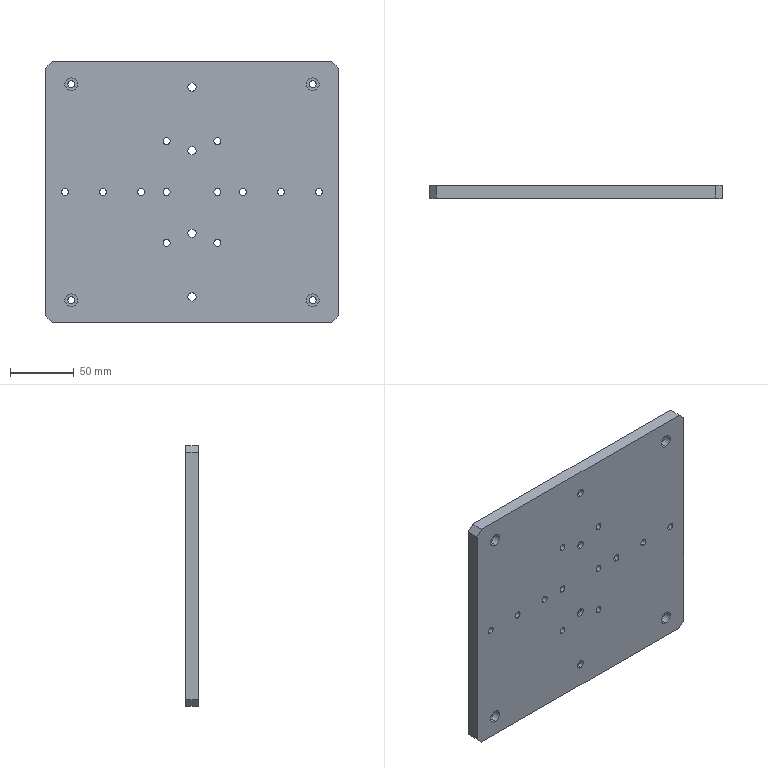Part | SolidWorks | features HoleWzd 3, Chamfer 1, Extrusion 1 | 1 solid | 110 faces | box 230 x 10 x 205 mm | volume 459180 mm3 | cylinder 80 | plane 30 | commonest cylinder face diameters 5.5 x32 10 x32 6.6 x8 11 x8